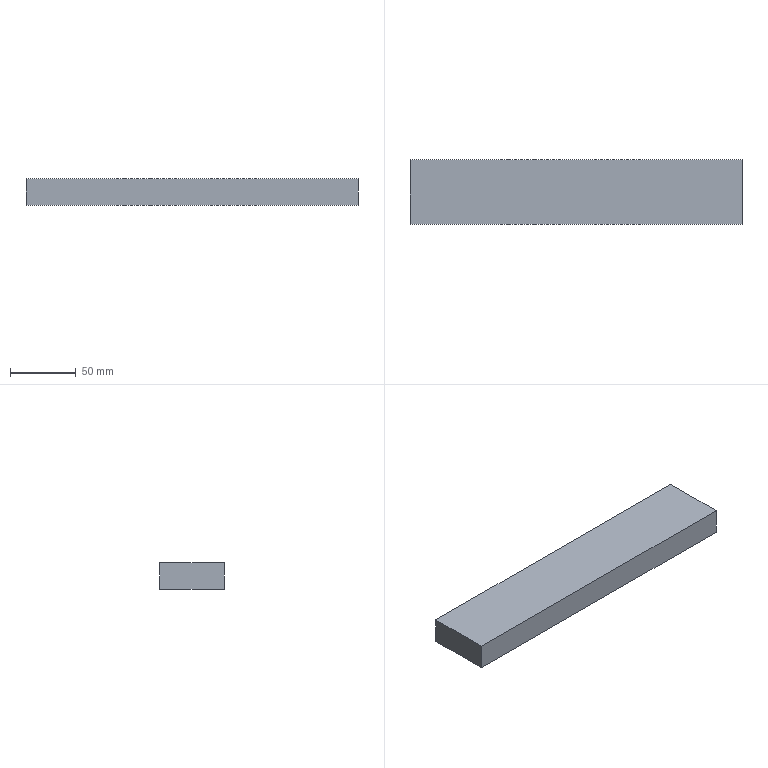Part | NX | features DATUM_CSYS 2, EXTRUDE 1, SKETCH 1 | 1 solid | 6 faces | box 252 x 49 x 20 mm | volume 246960 mm3 | plane 6
STEP:
#1=CARTESIAN_POINT('',(-126.,24.5,0.));
#2=VERTEX_POINT('',#1);
#3=CARTESIAN_POINT('',(126.,24.5,0.));
#4=VERTEX_POINT('',#3);
#5=CARTESIAN_POINT('',(-126.,24.5,0.));
#6=DIRECTION('',(1.,0.,0.));
#7=VECTOR('',#6,1000.);
#8=LINE('',#5,#7);
#9=EDGE_CURVE('',#2,#4,#8,.T.);
#10=ORIENTED_EDGE('',*,*,#9,.F.);
#11=CARTESIAN_POINT('',(-126.,24.5,20.));
#12=VERTEX_POINT('',#11);
#13=CARTESIAN_POINT('',(-126.,24.5,20.));
#14=DIRECTION('',(0.,0.,-1.));
#15=VECTOR('',#14,1000.);
#16=LINE('',#13,#15);
#17=EDGE_CURVE('',#12,#2,#16,.T.);
#18=ORIENTED_EDGE('',*,*,#17,.F.);
#19=CARTESIAN_POINT('',(126.,24.5,20.));
#20=VERTEX_POINT('',#19);
#21=CARTESIAN_POINT('',(-126.,24.5,20.));
#22=DIRECTION('',(1.,0.,0.));
#23=VECTOR('',#22,1000.);
#24=LINE('',#21,#23);
#25=EDGE_CURVE('',#12,#20,#24,.T.);
#26=ORIENTED_EDGE('',*,*,#25,.T.);
#27=CARTESIAN_POINT('',(126.,24.5,20.));
#28=DIRECTION('',(0.,0.,-1.));
#29=VECTOR('',#28,1000.);
#30=LINE('',#27,#29);
#31=EDGE_CURVE('',#20,#4,#30,.T.);
#32=ORIENTED_EDGE('',*,*,#31,.T.);
#33=EDGE_LOOP('',(#10,#18,#26,#32));
#34=FACE_BOUND('',#33,.T.);
#35=CARTESIAN_POINT('',(-126.,24.5,20.));
#36=DIRECTION('',(0.,1.,0.));
#37=DIRECTION('',(0.,0.,1.));
#38=AXIS2_PLACEMENT_3D('',#35,#36,#37);
#39=PLANE('',#38);
#40=ADVANCED_FACE('',(#34),#39,.T.);
#41=CARTESIAN_POINT('',(126.,-24.5,0.));
#42=VERTEX_POINT('',#41);
#43=CARTESIAN_POINT('',(126.,24.5,0.));
#44=DIRECTION('',(0.,-1.,0.));
#45=VECTOR('',#44,1000.);
#46=LINE('',#43,#45);
#47=EDGE_CURVE('',#4,#42,#46,.T.);
#48=ORIENTED_EDGE('',*,*,#47,.F.);
#49=ORIENTED_EDGE('',*,*,#31,.F.);
#50=CARTESIAN_POINT('',(126.,-24.5,20.));
#51=VERTEX_POINT('',#50);
#52=CARTESIAN_POINT('',(126.,24.5,20.));
#53=DIRECTION('',(0.,-1.,0.));
#54=VECTOR('',#53,1000.);
#55=LINE('',#52,#54);
#56=EDGE_CURVE('',#20,#51,#55,.T.);
#57=ORIENTED_EDGE('',*,*,#56,.T.);
#58=CARTESIAN_POINT('',(126.,-24.5,20.));
#59=DIRECTION('',(0.,0.,-1.));
#60=VECTOR('',#59,1000.);
#61=LINE('',#58,#60);
#62=EDGE_CURVE('',#51,#42,#61,.T.);
#63=ORIENTED_EDGE('',*,*,#62,.T.);
#64=EDGE_LOOP('',(#48,#49,#57,#63));
#65=FACE_BOUND('',#64,.T.);
#66=CARTESIAN_POINT('',(126.,24.5,20.));
#67=DIRECTION('',(1.,0.,0.));
#68=DIRECTION('',(0.,0.,-1.));
#69=AXIS2_PLACEMENT_3D('',#66,#67,#68);
#70=PLANE('',#69);
#71=ADVANCED_FACE('',(#65),#70,.T.);
#72=CARTESIAN_POINT('',(-126.,-24.5,0.));
#73=VERTEX_POINT('',#72);
#74=CARTESIAN_POINT('',(126.,-24.5,0.));
#75=DIRECTION('',(-1.,0.,0.));
#76=VECTOR('',#75,1000.);
#77=LINE('',#74,#76);
#78=EDGE_CURVE('',#42,#73,#77,.T.);
#79=ORIENTED_EDGE('',*,*,#78,.F.);
#80=ORIENTED_EDGE('',*,*,#62,.F.);
#81=CARTESIAN_POINT('',(-126.,-24.5,20.));
#82=VERTEX_POINT('',#81);
#83=CARTESIAN_POINT('',(126.,-24.5,20.));
#84=DIRECTION('',(-1.,0.,0.));
#85=VECTOR('',#84,1000.);
#86=LINE('',#83,#85);
#87=EDGE_CURVE('',#51,#82,#86,.T.);
#88=ORIENTED_EDGE('',*,*,#87,.T.);
#89=CARTESIAN_POINT('',(-126.,-24.5,20.));
#90=DIRECTION('',(0.,0.,-1.));
#91=VECTOR('',#90,1000.);
#92=LINE('',#89,#91);
#93=EDGE_CURVE('',#82,#73,#92,.T.);
#94=ORIENTED_EDGE('',*,*,#93,.T.);
#95=EDGE_LOOP('',(#79,#80,#88,#94));
#96=FACE_BOUND('',#95,.T.);
#97=CARTESIAN_POINT('',(126.,-24.5,20.));
#98=DIRECTION('',(0.,-1.,0.));
#99=DIRECTION('',(0.,0.,-1.));
#100=AXIS2_PLACEMENT_3D('',#97,#98,#99);
#101=PLANE('',#100);
#102=ADVANCED_FACE('',(#96),#101,.T.);
#103=CARTESIAN_POINT('',(-126.,-24.5,0.));
#104=DIRECTION('',(0.,1.,0.));
#105=VECTOR('',#104,1000.);
#106=LINE('',#103,#105);
#107=EDGE_CURVE('',#73,#2,#106,.T.);
#108=ORIENTED_EDGE('',*,*,#107,.F.);
#109=ORIENTED_EDGE('',*,*,#93,.F.);
#110=CARTESIAN_POINT('',(-126.,-24.5,20.));
#111=DIRECTION('',(0.,1.,0.));
#112=VECTOR('',#111,1000.);
#113=LINE('',#110,#112);
#114=EDGE_CURVE('',#82,#12,#113,.T.);
#115=ORIENTED_EDGE('',*,*,#114,.T.);
#116=ORIENTED_EDGE('',*,*,#17,.T.);
#117=EDGE_LOOP('',(#108,#109,#115,#116));
#118=FACE_BOUND('',#117,.T.);
#119=CARTESIAN_POINT('',(-126.,-24.5,20.));
#120=DIRECTION('',(-1.,0.,0.));
#121=DIRECTION('',(0.,0.,1.));
#122=AXIS2_PLACEMENT_3D('',#119,#120,#121);
#123=PLANE('',#122);
#124=ADVANCED_FACE('',(#118),#123,.T.);
#125=ORIENTED_EDGE('',*,*,#25,.F.);
#126=ORIENTED_EDGE('',*,*,#114,.F.);
#127=ORIENTED_EDGE('',*,*,#87,.F.);
#128=ORIENTED_EDGE('',*,*,#56,.F.);
#129=EDGE_LOOP('',(#125,#126,#127,#128));
#130=FACE_BOUND('',#129,.T.);
#131=CARTESIAN_POINT('',(0.,0.,20.));
#132=DIRECTION('',(0.,0.,-1.));
#133=DIRECTION('',(-1.,0.,0.));
#134=AXIS2_PLACEMENT_3D('',#131,#132,#133);
#135=PLANE('',#134);
#136=ADVANCED_FACE('',(#130),#135,.F.);
#137=ORIENTED_EDGE('',*,*,#9,.T.);
#138=ORIENTED_EDGE('',*,*,#47,.T.);
#139=ORIENTED_EDGE('',*,*,#78,.T.);
#140=ORIENTED_EDGE('',*,*,#107,.T.);
#141=EDGE_LOOP('',(#137,#138,#139,#140));
#142=FACE_BOUND('',#141,.T.);
#143=CARTESIAN_POINT('',(0.,0.,0.));
#144=DIRECTION('',(0.,0.,-1.));
#145=DIRECTION('',(-1.,0.,0.));
#146=AXIS2_PLACEMENT_3D('',#143,#144,#145);
#147=PLANE('',#146);
#148=ADVANCED_FACE('',(#142),#147,.T.);
#149=CLOSED_SHELL('',(#40,#71,#102,#124,#136,#148));
#150=MANIFOLD_SOLID_BREP('',#149);
#151=(LENGTH_UNIT()NAMED_UNIT(*)SI_UNIT(.MILLI.,.METRE.));
#152=UNCERTAINTY_MEASURE_WITH_UNIT(LENGTH_MEASURE(0.00001),#151,'','');
#153=(NAMED_UNIT(*)PLANE_ANGLE_UNIT()SI_UNIT($,.RADIAN.));
#154=(NAMED_UNIT(*)SI_UNIT($,.STERADIAN.)SOLID_ANGLE_UNIT());
#155=(GEOMETRIC_REPRESENTATION_CONTEXT(3)GLOBAL_UNCERTAINTY_ASSIGNED_CONTEXT((#152))GLOBAL_UNIT_ASSIGNED_CONTEXT((#151,#153,#154))REPRESENTATION_CONTEXT('',''));
#156=ADVANCED_BREP_SHAPE_REPRESENTATION('',(#150),#155);